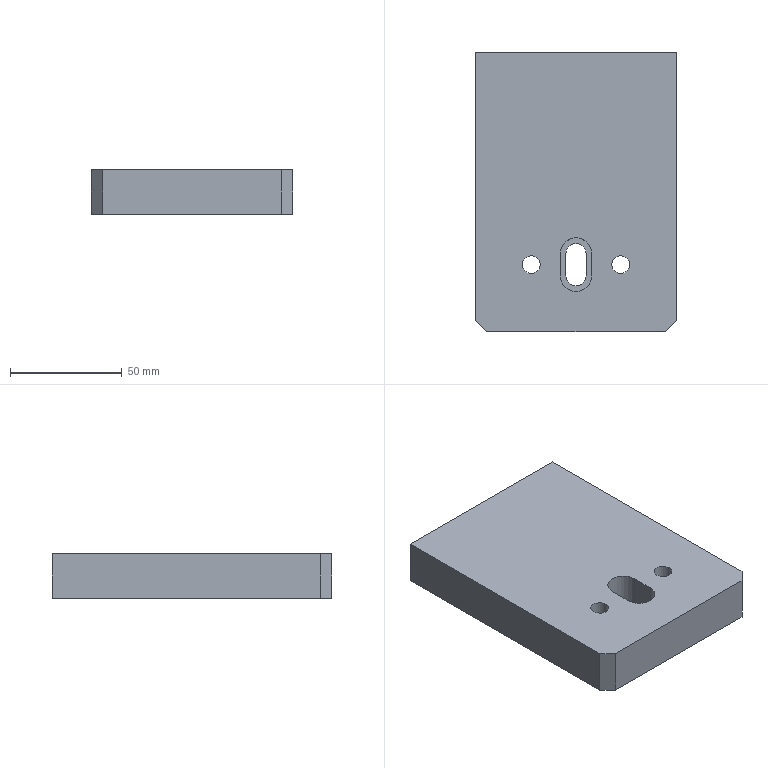Part | NX | features solid 2 | 1 solid | 19 faces | box 90 x 125 x 20 mm | volume 217523 mm3 | plane 13 | cylinder 6 | commonest cylinder face diameters 8 x2 9 x2 14 x2
STEP:
#1=CARTESIAN_POINT('',(-1205.,-500.,-85.));
#2=VERTEX_POINT('',#1);
#3=CARTESIAN_POINT('',(-1205.,-620.,-85.));
#4=VERTEX_POINT('',#3);
#5=CARTESIAN_POINT('',(-1205.,-582.007,-85.));
#6=DIRECTION('',(0.,-1.,0.));
#7=VECTOR('',#6,1000.);
#8=LINE('',#5,#7);
#9=EDGE_CURVE('',#2,#4,#8,.T.);
#10=ORIENTED_EDGE('',*,*,#9,.F.);
#11=CARTESIAN_POINT('',(-1205.,-500.,-105.));
#12=VERTEX_POINT('',#11);
#13=CARTESIAN_POINT('',(-1205.,-500.,-100.));
#14=DIRECTION('',(0.,0.,-1.));
#15=VECTOR('',#14,1000.);
#16=LINE('',#13,#15);
#17=EDGE_CURVE('',#2,#12,#16,.T.);
#18=ORIENTED_EDGE('',*,*,#17,.T.);
#19=CARTESIAN_POINT('',(-1205.,-620.,-105.));
#20=VERTEX_POINT('',#19);
#21=CARTESIAN_POINT('',(-1205.,-534.,-105.));
#22=DIRECTION('',(0.,-1.,0.));
#23=VECTOR('',#22,1000.);
#24=LINE('',#21,#23);
#25=EDGE_CURVE('',#12,#20,#24,.T.);
#26=ORIENTED_EDGE('',*,*,#25,.T.);
#27=CARTESIAN_POINT('',(-1205.,-620.,-100.));
#28=DIRECTION('',(0.,0.,-1.));
#29=VECTOR('',#28,1000.);
#30=LINE('',#27,#29);
#31=EDGE_CURVE('',#4,#20,#30,.T.);
#32=ORIENTED_EDGE('',*,*,#31,.F.);
#33=EDGE_LOOP('',(#10,#18,#26,#32));
#34=FACE_BOUND('',#33,.T.);
#35=CARTESIAN_POINT('',(-1205.,-545.,-100.));
#36=DIRECTION('',(-1.,0.,0.));
#37=DIRECTION('',(0.,-1.,0.));
#38=AXIS2_PLACEMENT_3D('',#35,#36,#37);
#39=PLANE('',#38);
#40=ADVANCED_FACE('',(#34),#39,.T.);
#41=CARTESIAN_POINT('',(-1115.,-500.,-105.));
#42=VERTEX_POINT('',#41);
#43=CARTESIAN_POINT('',(-1115.,-620.,-105.));
#44=VERTEX_POINT('',#43);
#45=CARTESIAN_POINT('',(-1115.,-545.,-105.));
#46=DIRECTION('',(0.,-1.,0.));
#47=VECTOR('',#46,1000.);
#48=LINE('',#45,#47);
#49=EDGE_CURVE('',#42,#44,#48,.T.);
#50=ORIENTED_EDGE('',*,*,#49,.F.);
#51=CARTESIAN_POINT('',(-1115.,-500.,-85.));
#52=VERTEX_POINT('',#51);
#53=CARTESIAN_POINT('',(-1115.,-500.,-100.));
#54=DIRECTION('',(0.,0.,1.));
#55=VECTOR('',#54,1000.);
#56=LINE('',#53,#55);
#57=EDGE_CURVE('',#42,#52,#56,.T.);
#58=ORIENTED_EDGE('',*,*,#57,.T.);
#59=CARTESIAN_POINT('',(-1115.,-620.,-85.));
#60=VERTEX_POINT('',#59);
#61=CARTESIAN_POINT('',(-1115.,-545.,-85.));
#62=DIRECTION('',(0.,-1.,0.));
#63=VECTOR('',#62,1000.);
#64=LINE('',#61,#63);
#65=EDGE_CURVE('',#52,#60,#64,.T.);
#66=ORIENTED_EDGE('',*,*,#65,.T.);
#67=CARTESIAN_POINT('',(-1115.,-620.,-100.));
#68=DIRECTION('',(0.,0.,1.));
#69=VECTOR('',#68,1000.);
#70=LINE('',#67,#69);
#71=EDGE_CURVE('',#44,#60,#70,.T.);
#72=ORIENTED_EDGE('',*,*,#71,.F.);
#73=EDGE_LOOP('',(#50,#58,#66,#72));
#74=FACE_BOUND('',#73,.T.);
#75=CARTESIAN_POINT('',(-1115.,-545.,-100.));
#76=DIRECTION('',(1.,0.,0.));
#77=DIRECTION('',(0.,0.,1.));
#78=AXIS2_PLACEMENT_3D('',#75,#76,#77);
#79=PLANE('',#78);
#80=ADVANCED_FACE('',(#74),#79,.T.);
#81=CARTESIAN_POINT('',(-1164.5,-590.,-105.));
#82=VERTEX_POINT('',#81);
#83=CARTESIAN_POINT('',(-1164.5,-600.,-105.));
#84=VERTEX_POINT('',#83);
#85=CARTESIAN_POINT('',(-1164.5,-534.,-105.));
#86=DIRECTION('',(0.,-1.,0.));
#87=VECTOR('',#86,1000.);
#88=LINE('',#85,#87);
#89=EDGE_CURVE('',#82,#84,#88,.T.);
#90=ORIENTED_EDGE('',*,*,#89,.T.);
#91=CARTESIAN_POINT('',(-1155.5,-600.,-105.));
#92=VERTEX_POINT('',#91);
#93=CARTESIAN_POINT('',(-1160.,-600.,-105.));
#94=DIRECTION('',(0.,0.,1.));
#95=DIRECTION('',(1.,0.,0.));
#96=AXIS2_PLACEMENT_3D('',#93,#94,#95);
#97=CIRCLE('',#96,4.5);
#98=EDGE_CURVE('',#84,#92,#97,.T.);
#99=ORIENTED_EDGE('',*,*,#98,.T.);
#100=CARTESIAN_POINT('',(-1155.5,-590.,-105.));
#101=VERTEX_POINT('',#100);
#102=CARTESIAN_POINT('',(-1155.5,-534.,-105.));
#103=DIRECTION('',(0.,-1.,0.));
#104=VECTOR('',#103,1000.);
#105=LINE('',#102,#104);
#106=EDGE_CURVE('',#101,#92,#105,.T.);
#107=ORIENTED_EDGE('',*,*,#106,.F.);
#108=CARTESIAN_POINT('',(-1160.,-590.,-105.));
#109=DIRECTION('',(0.,0.,1.));
#110=DIRECTION('',(1.,0.,0.));
#111=AXIS2_PLACEMENT_3D('',#108,#109,#110);
#112=CIRCLE('',#111,4.5);
#113=EDGE_CURVE('',#101,#82,#112,.T.);
#114=ORIENTED_EDGE('',*,*,#113,.T.);
#115=EDGE_LOOP('',(#90,#99,#107,#114));
#116=FACE_BOUND('',#115,.T.);
#117=CARTESIAN_POINT('',(-1176.,-595.,-105.));
#118=VERTEX_POINT('',#117);
#119=CARTESIAN_POINT('',(-1180.,-595.,-105.));
#120=DIRECTION('',(0.,0.,1.));
#121=DIRECTION('',(1.,0.,0.));
#122=AXIS2_PLACEMENT_3D('',#119,#120,#121);
#123=CIRCLE('',#122,4.);
#124=EDGE_CURVE('',#118,#118,#123,.T.);
#125=ORIENTED_EDGE('',*,*,#124,.T.);
#126=EDGE_LOOP('',(#125));
#127=FACE_BOUND('',#126,.T.);
#128=CARTESIAN_POINT('',(-1136.,-595.,-105.));
#129=VERTEX_POINT('',#128);
#130=CARTESIAN_POINT('',(-1140.,-595.,-105.));
#131=DIRECTION('',(0.,0.,1.));
#132=DIRECTION('',(1.,0.,0.));
#133=AXIS2_PLACEMENT_3D('',#130,#131,#132);
#134=CIRCLE('',#133,4.);
#135=EDGE_CURVE('',#129,#129,#134,.T.);
#136=ORIENTED_EDGE('',*,*,#135,.T.);
#137=EDGE_LOOP('',(#136));
#138=FACE_BOUND('',#137,.T.);
#139=CARTESIAN_POINT('',(-1185.,-500.,-105.));
#140=DIRECTION('',(-1.,0.,0.));
#141=VECTOR('',#140,1000.);
#142=LINE('',#139,#141);
#143=EDGE_CURVE('',#42,#12,#142,.T.);
#144=ORIENTED_EDGE('',*,*,#143,.F.);
#145=ORIENTED_EDGE('',*,*,#49,.T.);
#146=CARTESIAN_POINT('',(-1120.,-625.,-105.));
#147=VERTEX_POINT('',#146);
#148=CARTESIAN_POINT('',(-1104.5,-609.5,-105.));
#149=DIRECTION('',(-0.7071,-0.7071,0.));
#150=VECTOR('',#149,1000.);
#151=LINE('',#148,#150);
#152=EDGE_CURVE('',#147,#44,#151,.F.);
#153=ORIENTED_EDGE('',*,*,#152,.F.);
#154=CARTESIAN_POINT('',(-1200.,-625.,-105.));
#155=VERTEX_POINT('',#154);
#156=CARTESIAN_POINT('',(-1000.,-625.,-105.));
#157=DIRECTION('',(-1.,0.,0.));
#158=VECTOR('',#157,1000.);
#159=LINE('',#156,#158);
#160=EDGE_CURVE('',#147,#155,#159,.T.);
#161=ORIENTED_EDGE('',*,*,#160,.T.);
#162=CARTESIAN_POINT('',(-1240.5,-584.5,-105.));
#163=DIRECTION('',(-0.7071,0.7071,0.));
#164=VECTOR('',#163,1000.);
#165=LINE('',#162,#164);
#166=EDGE_CURVE('',#20,#155,#165,.F.);
#167=ORIENTED_EDGE('',*,*,#166,.F.);
#168=ORIENTED_EDGE('',*,*,#25,.F.);
#169=EDGE_LOOP('',(#144,#145,#153,#161,#167,#168));
#170=FACE_BOUND('',#169,.T.);
#171=CARTESIAN_POINT('',(-1185.,-534.,-105.));
#172=DIRECTION('',(0.,0.,1.));
#173=DIRECTION('',(0.,-1.,0.));
#174=AXIS2_PLACEMENT_3D('',#171,#172,#173);
#175=PLANE('',#174);
#176=ADVANCED_FACE('',(#116,#127,#138,#170),#175,.F.);
#177=CARTESIAN_POINT('',(-1200.,-625.,-85.));
#178=VERTEX_POINT('',#177);
#179=CARTESIAN_POINT('',(-1120.,-625.,-85.));
#180=VERTEX_POINT('',#179);
#181=CARTESIAN_POINT('',(-1379.986,-625.,-85.));
#182=DIRECTION('',(1.,0.,0.));
#183=VECTOR('',#182,1000.);
#184=LINE('',#181,#183);
#185=EDGE_CURVE('',#178,#180,#184,.T.);
#186=ORIENTED_EDGE('',*,*,#185,.T.);
#187=CARTESIAN_POINT('',(-1120.,-625.,-85.));
#188=DIRECTION('',(0.7071,0.7071,0.));
#189=VECTOR('',#188,1000.);
#190=LINE('',#187,#189);
#191=EDGE_CURVE('',#60,#180,#190,.F.);
#192=ORIENTED_EDGE('',*,*,#191,.F.);
#193=ORIENTED_EDGE('',*,*,#65,.F.);
#194=CARTESIAN_POINT('',(-1379.986,-500.,-85.));
#195=DIRECTION('',(-1.,0.,0.));
#196=VECTOR('',#195,1000.);
#197=LINE('',#194,#196);
#198=EDGE_CURVE('',#52,#2,#197,.T.);
#199=ORIENTED_EDGE('',*,*,#198,.T.);
#200=ORIENTED_EDGE('',*,*,#9,.T.);
#201=CARTESIAN_POINT('',(-1205.,-620.,-85.));
#202=DIRECTION('',(0.7071,-0.7071,0.));
#203=VECTOR('',#202,1000.);
#204=LINE('',#201,#203);
#205=EDGE_CURVE('',#178,#4,#204,.F.);
#206=ORIENTED_EDGE('',*,*,#205,.F.);
#207=EDGE_LOOP('',(#186,#192,#193,#199,#200,#206));
#208=FACE_BOUND('',#207,.T.);
#209=CARTESIAN_POINT('',(-1136.,-595.,-85.));
#210=VERTEX_POINT('',#209);
#211=CARTESIAN_POINT('',(-1140.,-595.,-85.));
#212=DIRECTION('',(0.,0.,1.));
#213=DIRECTION('',(1.,0.,0.));
#214=AXIS2_PLACEMENT_3D('',#211,#212,#213);
#215=CIRCLE('',#214,4.);
#216=EDGE_CURVE('',#210,#210,#215,.F.);
#217=ORIENTED_EDGE('',*,*,#216,.T.);
#218=EDGE_LOOP('',(#217));
#219=FACE_BOUND('',#218,.T.);
#220=CARTESIAN_POINT('',(-1176.,-595.,-85.));
#221=VERTEX_POINT('',#220);
#222=CARTESIAN_POINT('',(-1180.,-595.,-85.));
#223=DIRECTION('',(0.,0.,1.));
#224=DIRECTION('',(1.,0.,0.));
#225=AXIS2_PLACEMENT_3D('',#222,#223,#224);
#226=CIRCLE('',#225,4.);
#227=EDGE_CURVE('',#221,#221,#226,.F.);
#228=ORIENTED_EDGE('',*,*,#227,.T.);
#229=EDGE_LOOP('',(#228));
#230=FACE_BOUND('',#229,.T.);
#231=CARTESIAN_POINT('',(-1153.,-600.,-85.));
#232=VERTEX_POINT('',#231);
#233=CARTESIAN_POINT('',(-1153.,-590.,-85.));
#234=VERTEX_POINT('',#233);
#235=CARTESIAN_POINT('',(-1153.,-602.,-85.));
#236=DIRECTION('',(0.,1.,0.));
#237=VECTOR('',#236,1000.);
#238=LINE('',#235,#237);
#239=EDGE_CURVE('',#232,#234,#238,.T.);
#240=ORIENTED_EDGE('',*,*,#239,.F.);
#241=CARTESIAN_POINT('',(-1167.,-600.,-85.));
#242=VERTEX_POINT('',#241);
#243=CARTESIAN_POINT('',(-1160.,-600.,-85.));
#244=DIRECTION('',(0.,0.,1.));
#245=DIRECTION('',(1.,0.,0.));
#246=AXIS2_PLACEMENT_3D('',#243,#244,#245);
#247=CIRCLE('',#246,7.);
#248=EDGE_CURVE('',#232,#242,#247,.F.);
#249=ORIENTED_EDGE('',*,*,#248,.T.);
#250=CARTESIAN_POINT('',(-1167.,-590.,-85.));
#251=VERTEX_POINT('',#250);
#252=CARTESIAN_POINT('',(-1167.,-602.,-85.));
#253=DIRECTION('',(0.,1.,0.));
#254=VECTOR('',#253,1000.);
#255=LINE('',#252,#254);
#256=EDGE_CURVE('',#242,#251,#255,.T.);
#257=ORIENTED_EDGE('',*,*,#256,.T.);
#258=CARTESIAN_POINT('',(-1160.,-590.,-85.));
#259=DIRECTION('',(0.,0.,1.));
#260=DIRECTION('',(1.,0.,0.));
#261=AXIS2_PLACEMENT_3D('',#258,#259,#260);
#262=CIRCLE('',#261,7.);
#263=EDGE_CURVE('',#251,#234,#262,.F.);
#264=ORIENTED_EDGE('',*,*,#263,.T.);
#265=EDGE_LOOP('',(#240,#249,#257,#264));
#266=FACE_BOUND('',#265,.T.);
#267=CARTESIAN_POINT('',(-1379.986,-582.007,-85.));
#268=DIRECTION('',(0.,0.,1.));
#269=DIRECTION('',(0.1736,-0.9848,0.));
#270=AXIS2_PLACEMENT_3D('',#267,#268,#269);
#271=PLANE('',#270);
#272=ADVANCED_FACE('',(#208,#219,#230,#266),#271,.T.);
#273=ORIENTED_EDGE('',*,*,#160,.F.);
#274=CARTESIAN_POINT('',(-1120.,-625.,-240.));
#275=DIRECTION('',(0.,0.,-1.));
#276=VECTOR('',#275,1000.);
#277=LINE('',#274,#276);
#278=EDGE_CURVE('',#180,#147,#277,.T.);
#279=ORIENTED_EDGE('',*,*,#278,.F.);
#280=ORIENTED_EDGE('',*,*,#185,.F.);
#281=CARTESIAN_POINT('',(-1200.,-625.,-240.));
#282=DIRECTION('',(0.,0.,1.));
#283=VECTOR('',#282,1000.);
#284=LINE('',#281,#283);
#285=EDGE_CURVE('',#155,#178,#284,.T.);
#286=ORIENTED_EDGE('',*,*,#285,.F.);
#287=EDGE_LOOP('',(#273,#279,#280,#286));
#288=FACE_BOUND('',#287,.T.);
#289=CARTESIAN_POINT('',(-1000.,-625.,-240.));
#290=DIRECTION('',(0.,-1.,0.));
#291=DIRECTION('',(1.,0.,0.));
#292=AXIS2_PLACEMENT_3D('',#289,#290,#291);
#293=PLANE('',#292);
#294=ADVANCED_FACE('',(#288),#293,.T.);
#295=CARTESIAN_POINT('',(-1155.5,-600.,-98.5));
#296=VERTEX_POINT('',#295);
#297=CARTESIAN_POINT('',(-1155.5,-590.,-98.5));
#298=VERTEX_POINT('',#297);
#299=CARTESIAN_POINT('',(-1155.5,-602.,-98.5));
#300=DIRECTION('',(0.,-1.,0.));
#301=VECTOR('',#300,1000.);
#302=LINE('',#299,#301);
#303=EDGE_CURVE('',#296,#298,#302,.F.);
#304=ORIENTED_EDGE('',*,*,#303,.F.);
#305=CARTESIAN_POINT('',(-1164.5,-600.,-98.5));
#306=VERTEX_POINT('',#305);
#307=CARTESIAN_POINT('',(-1160.,-600.,-98.5));
#308=DIRECTION('',(0.,0.,1.));
#309=DIRECTION('',(1.,0.,0.));
#310=AXIS2_PLACEMENT_3D('',#307,#308,#309);
#311=CIRCLE('',#310,4.5);
#312=EDGE_CURVE('',#296,#306,#311,.F.);
#313=ORIENTED_EDGE('',*,*,#312,.T.);
#314=CARTESIAN_POINT('',(-1164.5,-590.,-98.5));
#315=VERTEX_POINT('',#314);
#316=CARTESIAN_POINT('',(-1164.5,-602.,-98.5));
#317=DIRECTION('',(0.,-1.,0.));
#318=VECTOR('',#317,1000.);
#319=LINE('',#316,#318);
#320=EDGE_CURVE('',#306,#315,#319,.F.);
#321=ORIENTED_EDGE('',*,*,#320,.T.);
#322=CARTESIAN_POINT('',(-1160.,-590.,-98.5));
#323=DIRECTION('',(0.,0.,1.));
#324=DIRECTION('',(1.,0.,0.));
#325=AXIS2_PLACEMENT_3D('',#322,#323,#324);
#326=CIRCLE('',#325,4.5);
#327=EDGE_CURVE('',#315,#298,#326,.F.);
#328=ORIENTED_EDGE('',*,*,#327,.T.);
#329=EDGE_LOOP('',(#304,#313,#321,#328));
#330=FACE_BOUND('',#329,.T.);
#331=CARTESIAN_POINT('',(-1167.,-600.,-98.5));
#332=VERTEX_POINT('',#331);
#333=CARTESIAN_POINT('',(-1167.,-590.,-98.5));
#334=VERTEX_POINT('',#333);
#335=CARTESIAN_POINT('',(-1167.,-602.,-98.5));
#336=DIRECTION('',(0.,-1.,0.));
#337=VECTOR('',#336,1000.);
#338=LINE('',#335,#337);
#339=EDGE_CURVE('',#332,#334,#338,.F.);
#340=ORIENTED_EDGE('',*,*,#339,.F.);
#341=CARTESIAN_POINT('',(-1153.,-600.,-98.5));
#342=VERTEX_POINT('',#341);
#343=CARTESIAN_POINT('',(-1160.,-600.,-98.5));
#344=DIRECTION('',(0.,0.,1.));
#345=DIRECTION('',(1.,0.,0.));
#346=AXIS2_PLACEMENT_3D('',#343,#344,#345);
#347=CIRCLE('',#346,7.);
#348=EDGE_CURVE('',#332,#342,#347,.T.);
#349=ORIENTED_EDGE('',*,*,#348,.T.);
#350=CARTESIAN_POINT('',(-1153.,-590.,-98.5));
#351=VERTEX_POINT('',#350);
#352=CARTESIAN_POINT('',(-1153.,-602.,-98.5));
#353=DIRECTION('',(0.,-1.,0.));
#354=VECTOR('',#353,1000.);
#355=LINE('',#352,#354);
#356=EDGE_CURVE('',#342,#351,#355,.F.);
#357=ORIENTED_EDGE('',*,*,#356,.T.);
#358=CARTESIAN_POINT('',(-1160.,-590.,-98.5));
#359=DIRECTION('',(0.,0.,1.));
#360=DIRECTION('',(1.,0.,0.));
#361=AXIS2_PLACEMENT_3D('',#358,#359,#360);
#362=CIRCLE('',#361,7.);
#363=EDGE_CURVE('',#351,#334,#362,.T.);
#364=ORIENTED_EDGE('',*,*,#363,.T.);
#365=EDGE_LOOP('',(#340,#349,#357,#364));
#366=FACE_BOUND('',#365,.T.);
#367=CARTESIAN_POINT('',(-1160.,-602.,-98.5));
#368=DIRECTION('',(0.,0.,1.));
#369=DIRECTION('',(0.,1.,0.));
#370=AXIS2_PLACEMENT_3D('',#367,#368,#369);
#371=PLANE('',#370);
#372=ADVANCED_FACE('',(#330,#366),#371,.T.);
#373=ORIENTED_EDGE('',*,*,#256,.F.);
#374=CARTESIAN_POINT('',(-1167.,-600.,-108.5));
#375=DIRECTION('',(0.,0.,1.));
#376=VECTOR('',#375,1000.);
#377=LINE('',#374,#376);
#378=EDGE_CURVE('',#242,#332,#377,.F.);
#379=ORIENTED_EDGE('',*,*,#378,.T.);
#380=ORIENTED_EDGE('',*,*,#339,.T.);
#381=CARTESIAN_POINT('',(-1167.,-590.,-100.));
#382=DIRECTION('',(0.,0.,-1.));
#383=VECTOR('',#382,1000.);
#384=LINE('',#381,#383);
#385=EDGE_CURVE('',#334,#251,#384,.F.);
#386=ORIENTED_EDGE('',*,*,#385,.T.);
#387=EDGE_LOOP('',(#373,#379,#380,#386));
#388=FACE_BOUND('',#387,.T.);
#389=CARTESIAN_POINT('',(-1167.,-602.,-100.));
#390=DIRECTION('',(-1.,0.,0.));
#391=DIRECTION('',(0.,-1.,0.));
#392=AXIS2_PLACEMENT_3D('',#389,#390,#391);
#393=PLANE('',#392);
#394=ADVANCED_FACE('',(#388),#393,.F.);
#395=ORIENTED_EDGE('',*,*,#356,.F.);
#396=CARTESIAN_POINT('',(-1153.,-600.,-100.));
#397=DIRECTION('',(0.,0.,1.));
#398=VECTOR('',#397,1000.);
#399=LINE('',#396,#398);
#400=EDGE_CURVE('',#342,#232,#399,.T.);
#401=ORIENTED_EDGE('',*,*,#400,.T.);
#402=ORIENTED_EDGE('',*,*,#239,.T.);
#403=CARTESIAN_POINT('',(-1153.,-590.,-100.));
#404=DIRECTION('',(0.,0.,-1.));
#405=VECTOR('',#404,1000.);
#406=LINE('',#403,#405);
#407=EDGE_CURVE('',#234,#351,#406,.T.);
#408=ORIENTED_EDGE('',*,*,#407,.T.);
#409=EDGE_LOOP('',(#395,#401,#402,#408));
#410=FACE_BOUND('',#409,.T.);
#411=CARTESIAN_POINT('',(-1153.,-602.,-100.));
#412=DIRECTION('',(-1.,0.,0.));
#413=DIRECTION('',(0.,-1.,0.));
#414=AXIS2_PLACEMENT_3D('',#411,#412,#413);
#415=PLANE('',#414);
#416=ADVANCED_FACE('',(#410),#415,.T.);
#417=ORIENTED_EDGE('',*,*,#348,.F.);
#418=ORIENTED_EDGE('',*,*,#378,.F.);
#419=ORIENTED_EDGE('',*,*,#248,.F.);
#420=ORIENTED_EDGE('',*,*,#400,.F.);
#421=EDGE_LOOP('',(#417,#418,#419,#420));
#422=FACE_BOUND('',#421,.T.);
#423=CARTESIAN_POINT('',(-1160.,-600.,-100.));
#424=DIRECTION('',(0.,0.,1.));
#425=DIRECTION('',(-1.,0.,0.));
#426=AXIS2_PLACEMENT_3D('',#423,#424,#425);
#427=CYLINDRICAL_SURFACE('',#426,7.);
#428=ADVANCED_FACE('',(#422),#427,.F.);
#429=ORIENTED_EDGE('',*,*,#407,.F.);
#430=ORIENTED_EDGE('',*,*,#263,.F.);
#431=ORIENTED_EDGE('',*,*,#385,.F.);
#432=ORIENTED_EDGE('',*,*,#363,.F.);
#433=EDGE_LOOP('',(#429,#430,#431,#432));
#434=FACE_BOUND('',#433,.T.);
#435=CARTESIAN_POINT('',(-1160.,-590.,-100.));
#436=DIRECTION('',(0.,0.,-1.));
#437=DIRECTION('',(1.,0.,0.));
#438=AXIS2_PLACEMENT_3D('',#435,#436,#437);
#439=CYLINDRICAL_SURFACE('',#438,7.);
#440=ADVANCED_FACE('',(#434),#439,.F.);
#441=CARTESIAN_POINT('',(-1164.5,-590.,-90.));
#442=DIRECTION('',(0.,0.,-1.));
#443=VECTOR('',#442,1000.);
#444=LINE('',#441,#443);
#445=EDGE_CURVE('',#315,#82,#444,.T.);
#446=ORIENTED_EDGE('',*,*,#445,.F.);
#447=ORIENTED_EDGE('',*,*,#320,.F.);
#448=CARTESIAN_POINT('',(-1164.5,-600.,-90.));
#449=DIRECTION('',(0.,0.,1.));
#450=VECTOR('',#449,1000.);
#451=LINE('',#448,#450);
#452=EDGE_CURVE('',#84,#306,#451,.T.);
#453=ORIENTED_EDGE('',*,*,#452,.F.);
#454=ORIENTED_EDGE('',*,*,#89,.F.);
#455=EDGE_LOOP('',(#446,#447,#453,#454));
#456=FACE_BOUND('',#455,.T.);
#457=CARTESIAN_POINT('',(-1164.5,-599.5,-90.));
#458=DIRECTION('',(-1.,0.,0.));
#459=DIRECTION('',(0.,-1.,0.));
#460=AXIS2_PLACEMENT_3D('',#457,#458,#459);
#461=PLANE('',#460);
#462=ADVANCED_FACE('',(#456),#461,.F.);
#463=ORIENTED_EDGE('',*,*,#106,.T.);
#464=CARTESIAN_POINT('',(-1155.5,-600.,-140.));
#465=DIRECTION('',(0.,0.,1.));
#466=VECTOR('',#465,1000.);
#467=LINE('',#464,#466);
#468=EDGE_CURVE('',#296,#92,#467,.F.);
#469=ORIENTED_EDGE('',*,*,#468,.F.);
#470=ORIENTED_EDGE('',*,*,#303,.T.);
#471=CARTESIAN_POINT('',(-1155.5,-590.,-90.));
#472=DIRECTION('',(0.,0.,-1.));
#473=VECTOR('',#472,1000.);
#474=LINE('',#471,#473);
#475=EDGE_CURVE('',#101,#298,#474,.F.);
#476=ORIENTED_EDGE('',*,*,#475,.F.);
#477=EDGE_LOOP('',(#463,#469,#470,#476));
#478=FACE_BOUND('',#477,.T.);
#479=CARTESIAN_POINT('',(-1155.5,-599.5,-90.));
#480=DIRECTION('',(-1.,0.,0.));
#481=DIRECTION('',(0.,-1.,0.));
#482=AXIS2_PLACEMENT_3D('',#479,#480,#481);
#483=PLANE('',#482);
#484=ADVANCED_FACE('',(#478),#483,.T.);
#485=ORIENTED_EDGE('',*,*,#452,.T.);
#486=ORIENTED_EDGE('',*,*,#312,.F.);
#487=ORIENTED_EDGE('',*,*,#468,.T.);
#488=ORIENTED_EDGE('',*,*,#98,.F.);
#489=EDGE_LOOP('',(#485,#486,#487,#488));
#490=FACE_BOUND('',#489,.T.);
#491=CARTESIAN_POINT('',(-1160.,-600.,-90.));
#492=DIRECTION('',(0.,0.,-1.));
#493=DIRECTION('',(1.,0.,0.));
#494=AXIS2_PLACEMENT_3D('',#491,#492,#493);
#495=CYLINDRICAL_SURFACE('',#494,4.5);
#496=ADVANCED_FACE('',(#490),#495,.F.);
#497=ORIENTED_EDGE('',*,*,#475,.T.);
#498=ORIENTED_EDGE('',*,*,#327,.F.);
#499=ORIENTED_EDGE('',*,*,#445,.T.);
#500=ORIENTED_EDGE('',*,*,#113,.F.);
#501=EDGE_LOOP('',(#497,#498,#499,#500));
#502=FACE_BOUND('',#501,.T.);
#503=CARTESIAN_POINT('',(-1160.,-590.,-90.));
#504=DIRECTION('',(0.,0.,1.));
#505=DIRECTION('',(-1.,0.,0.));
#506=AXIS2_PLACEMENT_3D('',#503,#504,#505);
#507=CYLINDRICAL_SURFACE('',#506,4.5);
#508=ADVANCED_FACE('',(#502),#507,.F.);
#509=ORIENTED_EDGE('',*,*,#227,.F.);
#510=EDGE_LOOP('',(#509));
#511=FACE_BOUND('',#510,.T.);
#512=ORIENTED_EDGE('',*,*,#124,.F.);
#513=EDGE_LOOP('',(#512));
#514=FACE_BOUND('',#513,.T.);
#515=CARTESIAN_POINT('',(-1180.,-595.,-100.));
#516=DIRECTION('',(0.,0.,-1.));
#517=DIRECTION('',(1.,0.,0.));
#518=AXIS2_PLACEMENT_3D('',#515,#516,#517);
#519=CYLINDRICAL_SURFACE('',#518,4.);
#520=ADVANCED_FACE('',(#511,#514),#519,.F.);
#521=ORIENTED_EDGE('',*,*,#216,.F.);
#522=EDGE_LOOP('',(#521));
#523=FACE_BOUND('',#522,.T.);
#524=ORIENTED_EDGE('',*,*,#135,.F.);
#525=EDGE_LOOP('',(#524));
#526=FACE_BOUND('',#525,.T.);
#527=CARTESIAN_POINT('',(-1140.,-595.,-100.));
#528=DIRECTION('',(0.,0.,-1.));
#529=DIRECTION('',(1.,0.,0.));
#530=AXIS2_PLACEMENT_3D('',#527,#528,#529);
#531=CYLINDRICAL_SURFACE('',#530,4.);
#532=ADVANCED_FACE('',(#523,#526),#531,.F.);
#533=ORIENTED_EDGE('',*,*,#205,.T.);
#534=ORIENTED_EDGE('',*,*,#31,.T.);
#535=ORIENTED_EDGE('',*,*,#166,.T.);
#536=ORIENTED_EDGE('',*,*,#285,.T.);
#537=EDGE_LOOP('',(#533,#534,#535,#536));
#538=FACE_BOUND('',#537,.T.);
#539=CARTESIAN_POINT('',(-1205.,-620.,-100.));
#540=DIRECTION('',(0.7071,0.7071,0.));
#541=DIRECTION('',(0.7071,-0.7071,0.));
#542=AXIS2_PLACEMENT_3D('',#539,#540,#541);
#543=PLANE('',#542);
#544=ADVANCED_FACE('',(#538),#543,.F.);
#545=ORIENTED_EDGE('',*,*,#191,.T.);
#546=ORIENTED_EDGE('',*,*,#278,.T.);
#547=ORIENTED_EDGE('',*,*,#152,.T.);
#548=ORIENTED_EDGE('',*,*,#71,.T.);
#549=EDGE_LOOP('',(#545,#546,#547,#548));
#550=FACE_BOUND('',#549,.T.);
#551=CARTESIAN_POINT('',(-1120.,-625.,-240.));
#552=DIRECTION('',(-0.7071,0.7071,0.));
#553=DIRECTION('',(0.7071,0.7071,0.));
#554=AXIS2_PLACEMENT_3D('',#551,#552,#553);
#555=PLANE('',#554);
#556=ADVANCED_FACE('',(#550),#555,.F.);
#557=ORIENTED_EDGE('',*,*,#17,.F.);
#558=ORIENTED_EDGE('',*,*,#198,.F.);
#559=ORIENTED_EDGE('',*,*,#57,.F.);
#560=ORIENTED_EDGE('',*,*,#143,.T.);
#561=EDGE_LOOP('',(#557,#558,#559,#560));
#562=FACE_BOUND('',#561,.T.);
#563=CARTESIAN_POINT('',(-1120.,-500.,-100.));
#564=DIRECTION('',(0.,1.,0.));
#565=DIRECTION('',(-1.,0.,0.));
#566=AXIS2_PLACEMENT_3D('',#563,#564,#565);
#567=PLANE('',#566);
#568=ADVANCED_FACE('',(#562),#567,.T.);
#569=CLOSED_SHELL('',(#40,#80,#176,#272,#294,#372,#394,#416,#428,#440,#462,#484,#496,#508,#520,#532,#544,#556,#568));
#570=MANIFOLD_SOLID_BREP('',#569);
#571=(LENGTH_UNIT()NAMED_UNIT(*)SI_UNIT(.MILLI.,.METRE.));
#572=UNCERTAINTY_MEASURE_WITH_UNIT(LENGTH_MEASURE(0.00001),#571,'','');
#573=(NAMED_UNIT(*)PLANE_ANGLE_UNIT()SI_UNIT($,.RADIAN.));
#574=(NAMED_UNIT(*)SI_UNIT($,.STERADIAN.)SOLID_ANGLE_UNIT());
#575=(GEOMETRIC_REPRESENTATION_CONTEXT(3)GLOBAL_UNCERTAINTY_ASSIGNED_CONTEXT((#572))GLOBAL_UNIT_ASSIGNED_CONTEXT((#571,#573,#574))REPRESENTATION_CONTEXT('',''));
#576=ADVANCED_BREP_SHAPE_REPRESENTATION('',(#570),#575);